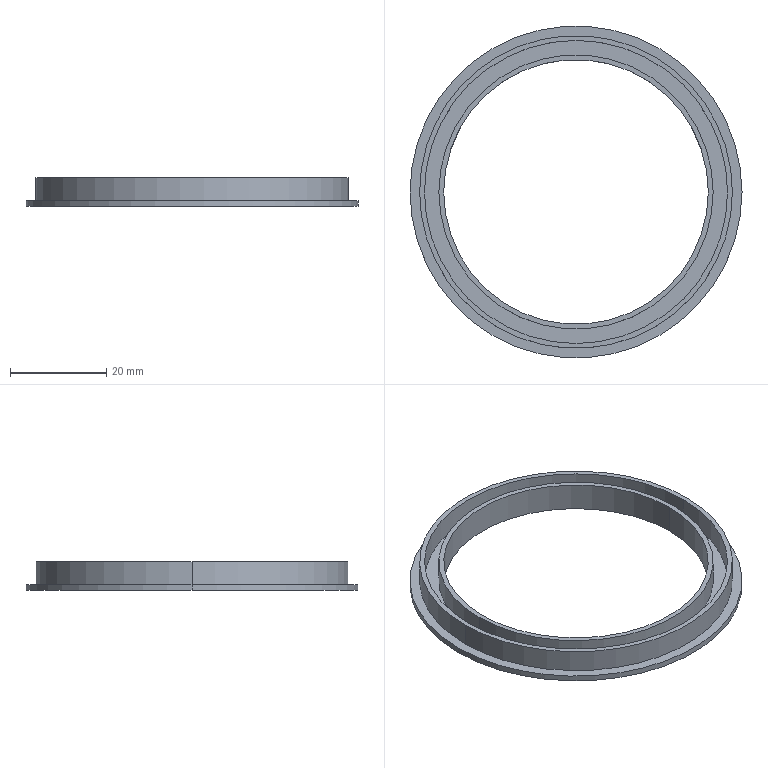Part | SolidWorks | features Extrusion 1, ICE 1 | 1 solid | 15 faces | box 69 x 69 x 6 mm | volume 3446 mm3 | cylinder 10 | plane 5 | commonest cylinder face diameters 55 x2 57 x2 63 x2 65 x2 69 x2
STEP:
#1=CARTESIAN_POINT('',(28.5,0.,6.));
#2=VERTEX_POINT('',#1);
#3=CARTESIAN_POINT('',(-28.5,0.,6.));
#4=VERTEX_POINT('',#3);
#5=CARTESIAN_POINT('',(0.,0.,6.));
#6=DIRECTION('',(0.,0.,1.));
#7=DIRECTION('',(1.,0.,0.));
#8=AXIS2_PLACEMENT_3D('',#5,#6,#7);
#9=CIRCLE('',#8,28.5);
#10=EDGE_CURVE('',#2,#4,#9,.T.);
#11=ORIENTED_EDGE('',*,*,#10,.F.);
#12=CARTESIAN_POINT('',(28.5,0.,1.2));
#13=VERTEX_POINT('',#12);
#14=CARTESIAN_POINT('',(28.5,0.,6.));
#15=DIRECTION('',(0.,0.,-1.));
#16=VECTOR('',#15,1000.);
#17=LINE('',#14,#16);
#18=EDGE_CURVE('',#2,#13,#17,.T.);
#19=ORIENTED_EDGE('',*,*,#18,.T.);
#20=CARTESIAN_POINT('',(-28.5,0.,1.2));
#21=VERTEX_POINT('',#20);
#22=CARTESIAN_POINT('',(0.,0.,1.2));
#23=DIRECTION('',(0.,0.,-1.));
#24=DIRECTION('',(1.,0.,0.));
#25=AXIS2_PLACEMENT_3D('',#22,#23,#24);
#26=CIRCLE('',#25,28.5);
#27=EDGE_CURVE('',#21,#13,#26,.T.);
#28=ORIENTED_EDGE('',*,*,#27,.F.);
#29=CARTESIAN_POINT('',(-28.5,0.,6.));
#30=DIRECTION('',(0.,0.,-1.));
#31=VECTOR('',#30,1000.);
#32=LINE('',#29,#31);
#33=EDGE_CURVE('',#4,#21,#32,.T.);
#34=ORIENTED_EDGE('',*,*,#33,.F.);
#35=EDGE_LOOP('',(#11,#19,#28,#34));
#36=FACE_OUTER_BOUND('',#35,.T.);
#37=CARTESIAN_POINT('',(0.,0.,6.));
#38=DIRECTION('',(0.,0.,-1.));
#39=DIRECTION('',(-1.,0.,0.));
#40=AXIS2_PLACEMENT_3D('',#37,#38,#39);
#41=CYLINDRICAL_SURFACE('',#40,28.5);
#42=ADVANCED_FACE('',(#36),#41,.T.);
#43=CARTESIAN_POINT('',(-27.5,0.,6.));
#44=VERTEX_POINT('',#43);
#45=CARTESIAN_POINT('',(27.5,0.,6.));
#46=VERTEX_POINT('',#45);
#47=CARTESIAN_POINT('',(0.,0.,6.));
#48=DIRECTION('',(0.,0.,1.));
#49=DIRECTION('',(1.,0.,0.));
#50=AXIS2_PLACEMENT_3D('',#47,#48,#49);
#51=CIRCLE('',#50,27.5);
#52=EDGE_CURVE('',#44,#46,#51,.T.);
#53=ORIENTED_EDGE('',*,*,#52,.T.);
#54=CARTESIAN_POINT('',(27.5,0.,0.));
#55=VERTEX_POINT('',#54);
#56=CARTESIAN_POINT('',(27.5,0.,1.2));
#57=DIRECTION('',(0.,0.,-1.));
#58=VECTOR('',#57,1000.);
#59=LINE('',#56,#58);
#60=EDGE_CURVE('',#46,#55,#59,.T.);
#61=ORIENTED_EDGE('',*,*,#60,.T.);
#62=CARTESIAN_POINT('',(-27.5,0.,0.));
#63=VERTEX_POINT('',#62);
#64=CARTESIAN_POINT('',(0.,0.,0.));
#65=DIRECTION('',(0.,0.,1.));
#66=DIRECTION('',(1.,0.,0.));
#67=AXIS2_PLACEMENT_3D('',#64,#65,#66);
#68=CIRCLE('',#67,27.5);
#69=EDGE_CURVE('',#63,#55,#68,.T.);
#70=ORIENTED_EDGE('',*,*,#69,.F.);
#71=CARTESIAN_POINT('',(-27.5,0.,1.2));
#72=DIRECTION('',(0.,0.,-1.));
#73=VECTOR('',#72,1000.);
#74=LINE('',#71,#73);
#75=EDGE_CURVE('',#44,#63,#74,.T.);
#76=ORIENTED_EDGE('',*,*,#75,.F.);
#77=EDGE_LOOP('',(#53,#61,#70,#76));
#78=FACE_OUTER_BOUND('',#77,.T.);
#79=CARTESIAN_POINT('',(0.,0.,1.2));
#80=DIRECTION('',(0.,0.,-1.));
#81=DIRECTION('',(-1.,0.,0.));
#82=AXIS2_PLACEMENT_3D('',#79,#80,#81);
#83=CYLINDRICAL_SURFACE('',#82,27.5);
#84=ADVANCED_FACE('',(#78),#83,.F.);
#85=CARTESIAN_POINT('',(34.5,0.,1.2));
#86=VERTEX_POINT('',#85);
#87=CARTESIAN_POINT('',(-34.5,0.,1.2));
#88=VERTEX_POINT('',#87);
#89=CARTESIAN_POINT('',(0.,0.,1.2));
#90=DIRECTION('',(0.,0.,1.));
#91=DIRECTION('',(1.,0.,0.));
#92=AXIS2_PLACEMENT_3D('',#89,#90,#91);
#93=CIRCLE('',#92,34.5);
#94=EDGE_CURVE('',#86,#88,#93,.T.);
#95=ORIENTED_EDGE('',*,*,#94,.F.);
#96=CARTESIAN_POINT('',(34.5,0.,0.));
#97=VERTEX_POINT('',#96);
#98=CARTESIAN_POINT('',(34.5,0.,1.2));
#99=DIRECTION('',(0.,0.,-1.));
#100=VECTOR('',#99,1000.);
#101=LINE('',#98,#100);
#102=EDGE_CURVE('',#86,#97,#101,.T.);
#103=ORIENTED_EDGE('',*,*,#102,.T.);
#104=CARTESIAN_POINT('',(-34.5,0.,0.));
#105=VERTEX_POINT('',#104);
#106=CARTESIAN_POINT('',(0.,0.,0.));
#107=DIRECTION('',(0.,0.,1.));
#108=DIRECTION('',(1.,0.,0.));
#109=AXIS2_PLACEMENT_3D('',#106,#107,#108);
#110=CIRCLE('',#109,34.5);
#111=EDGE_CURVE('',#97,#105,#110,.T.);
#112=ORIENTED_EDGE('',*,*,#111,.T.);
#113=CARTESIAN_POINT('',(-34.5,0.,1.2));
#114=DIRECTION('',(0.,0.,-1.));
#115=VECTOR('',#114,1000.);
#116=LINE('',#113,#115);
#117=EDGE_CURVE('',#88,#105,#116,.T.);
#118=ORIENTED_EDGE('',*,*,#117,.F.);
#119=EDGE_LOOP('',(#95,#103,#112,#118));
#120=FACE_OUTER_BOUND('',#119,.T.);
#121=CARTESIAN_POINT('',(0.,0.,1.2));
#122=DIRECTION('',(0.,0.,-1.));
#123=DIRECTION('',(-1.,0.,0.));
#124=AXIS2_PLACEMENT_3D('',#121,#122,#123);
#125=CYLINDRICAL_SURFACE('',#124,34.5);
#126=ADVANCED_FACE('',(#120),#125,.T.);
#127=CARTESIAN_POINT('',(32.5,0.,6.));
#128=VERTEX_POINT('',#127);
#129=CARTESIAN_POINT('',(-32.5,0.,6.));
#130=VERTEX_POINT('',#129);
#131=CARTESIAN_POINT('',(0.,0.,6.));
#132=DIRECTION('',(0.,0.,1.));
#133=DIRECTION('',(1.,0.,0.));
#134=AXIS2_PLACEMENT_3D('',#131,#132,#133);
#135=CIRCLE('',#134,32.5);
#136=EDGE_CURVE('',#128,#130,#135,.T.);
#137=ORIENTED_EDGE('',*,*,#136,.F.);
#138=CARTESIAN_POINT('',(32.5,0.,1.2));
#139=VERTEX_POINT('',#138);
#140=CARTESIAN_POINT('',(32.5,0.,6.));
#141=DIRECTION('',(0.,0.,-1.));
#142=VECTOR('',#141,1000.);
#143=LINE('',#140,#142);
#144=EDGE_CURVE('',#128,#139,#143,.T.);
#145=ORIENTED_EDGE('',*,*,#144,.T.);
#146=CARTESIAN_POINT('',(-32.5,0.,1.2));
#147=VERTEX_POINT('',#146);
#148=CARTESIAN_POINT('',(0.,0.,1.2));
#149=DIRECTION('',(0.,0.,1.));
#150=DIRECTION('',(1.,0.,0.));
#151=AXIS2_PLACEMENT_3D('',#148,#149,#150);
#152=CIRCLE('',#151,32.5);
#153=EDGE_CURVE('',#139,#147,#152,.T.);
#154=ORIENTED_EDGE('',*,*,#153,.T.);
#155=CARTESIAN_POINT('',(-32.5,0.,6.));
#156=DIRECTION('',(0.,0.,-1.));
#157=VECTOR('',#156,1000.);
#158=LINE('',#155,#157);
#159=EDGE_CURVE('',#130,#147,#158,.T.);
#160=ORIENTED_EDGE('',*,*,#159,.F.);
#161=EDGE_LOOP('',(#137,#145,#154,#160));
#162=FACE_OUTER_BOUND('',#161,.T.);
#163=CARTESIAN_POINT('',(0.,0.,6.));
#164=DIRECTION('',(0.,0.,-1.));
#165=DIRECTION('',(-1.,0.,0.));
#166=AXIS2_PLACEMENT_3D('',#163,#164,#165);
#167=CYLINDRICAL_SURFACE('',#166,32.5);
#168=ADVANCED_FACE('',(#162),#167,.T.);
#169=CARTESIAN_POINT('',(-31.5,0.,6.));
#170=VERTEX_POINT('',#169);
#171=CARTESIAN_POINT('',(31.5,0.,6.));
#172=VERTEX_POINT('',#171);
#173=CARTESIAN_POINT('',(0.,0.,6.));
#174=DIRECTION('',(0.,0.,1.));
#175=DIRECTION('',(1.,0.,0.));
#176=AXIS2_PLACEMENT_3D('',#173,#174,#175);
#177=CIRCLE('',#176,31.5);
#178=EDGE_CURVE('',#170,#172,#177,.T.);
#179=ORIENTED_EDGE('',*,*,#178,.T.);
#180=CARTESIAN_POINT('',(31.5,0.,1.2));
#181=VERTEX_POINT('',#180);
#182=CARTESIAN_POINT('',(31.5,0.,6.));
#183=DIRECTION('',(0.,0.,-1.));
#184=VECTOR('',#183,1000.);
#185=LINE('',#182,#184);
#186=EDGE_CURVE('',#172,#181,#185,.T.);
#187=ORIENTED_EDGE('',*,*,#186,.T.);
#188=CARTESIAN_POINT('',(-31.5,0.,1.2));
#189=VERTEX_POINT('',#188);
#190=CARTESIAN_POINT('',(0.,0.,1.2));
#191=DIRECTION('',(0.,0.,1.));
#192=DIRECTION('',(1.,0.,0.));
#193=AXIS2_PLACEMENT_3D('',#190,#191,#192);
#194=CIRCLE('',#193,31.5);
#195=EDGE_CURVE('',#189,#181,#194,.T.);
#196=ORIENTED_EDGE('',*,*,#195,.F.);
#197=CARTESIAN_POINT('',(-31.5,0.,6.));
#198=DIRECTION('',(0.,0.,-1.));
#199=VECTOR('',#198,1000.);
#200=LINE('',#197,#199);
#201=EDGE_CURVE('',#170,#189,#200,.T.);
#202=ORIENTED_EDGE('',*,*,#201,.F.);
#203=EDGE_LOOP('',(#179,#187,#196,#202));
#204=FACE_OUTER_BOUND('',#203,.T.);
#205=CARTESIAN_POINT('',(0.,0.,6.));
#206=DIRECTION('',(0.,0.,-1.));
#207=DIRECTION('',(-1.,0.,0.));
#208=AXIS2_PLACEMENT_3D('',#205,#206,#207);
#209=CYLINDRICAL_SURFACE('',#208,31.5);
#210=ADVANCED_FACE('',(#204),#209,.F.);
#211=ORIENTED_EDGE('',*,*,#186,.F.);
#212=CARTESIAN_POINT('',(0.,0.,6.));
#213=DIRECTION('',(0.,0.,1.));
#214=DIRECTION('',(1.,0.,0.));
#215=AXIS2_PLACEMENT_3D('',#212,#213,#214);
#216=CIRCLE('',#215,31.5);
#217=EDGE_CURVE('',#172,#170,#216,.T.);
#218=ORIENTED_EDGE('',*,*,#217,.T.);
#219=ORIENTED_EDGE('',*,*,#201,.T.);
#220=CARTESIAN_POINT('',(0.,0.,1.2));
#221=DIRECTION('',(0.,0.,1.));
#222=DIRECTION('',(1.,0.,0.));
#223=AXIS2_PLACEMENT_3D('',#220,#221,#222);
#224=CIRCLE('',#223,31.5);
#225=EDGE_CURVE('',#181,#189,#224,.T.);
#226=ORIENTED_EDGE('',*,*,#225,.F.);
#227=EDGE_LOOP('',(#211,#218,#219,#226));
#228=FACE_OUTER_BOUND('',#227,.T.);
#229=CARTESIAN_POINT('',(0.,0.,6.));
#230=DIRECTION('',(0.,0.,-1.));
#231=DIRECTION('',(-1.,0.,0.));
#232=AXIS2_PLACEMENT_3D('',#229,#230,#231);
#233=CYLINDRICAL_SURFACE('',#232,31.5);
#234=ADVANCED_FACE('',(#228),#233,.F.);
#235=ORIENTED_EDGE('',*,*,#144,.F.);
#236=CARTESIAN_POINT('',(0.,0.,6.));
#237=DIRECTION('',(0.,0.,1.));
#238=DIRECTION('',(1.,0.,0.));
#239=AXIS2_PLACEMENT_3D('',#236,#237,#238);
#240=CIRCLE('',#239,32.5);
#241=EDGE_CURVE('',#130,#128,#240,.T.);
#242=ORIENTED_EDGE('',*,*,#241,.F.);
#243=ORIENTED_EDGE('',*,*,#159,.T.);
#244=CARTESIAN_POINT('',(0.,0.,1.2));
#245=DIRECTION('',(0.,0.,1.));
#246=DIRECTION('',(1.,0.,0.));
#247=AXIS2_PLACEMENT_3D('',#244,#245,#246);
#248=CIRCLE('',#247,32.5);
#249=EDGE_CURVE('',#147,#139,#248,.T.);
#250=ORIENTED_EDGE('',*,*,#249,.T.);
#251=EDGE_LOOP('',(#235,#242,#243,#250));
#252=FACE_OUTER_BOUND('',#251,.T.);
#253=CARTESIAN_POINT('',(0.,0.,6.));
#254=DIRECTION('',(0.,0.,-1.));
#255=DIRECTION('',(-1.,0.,0.));
#256=AXIS2_PLACEMENT_3D('',#253,#254,#255);
#257=CYLINDRICAL_SURFACE('',#256,32.5);
#258=ADVANCED_FACE('',(#252),#257,.T.);
#259=ORIENTED_EDGE('',*,*,#178,.F.);
#260=ORIENTED_EDGE('',*,*,#217,.F.);
#261=EDGE_LOOP('',(#259,#260));
#262=FACE_BOUND('',#261,.T.);
#263=ORIENTED_EDGE('',*,*,#241,.T.);
#264=ORIENTED_EDGE('',*,*,#136,.T.);
#265=EDGE_LOOP('',(#263,#264));
#266=FACE_OUTER_BOUND('',#265,.T.);
#267=CARTESIAN_POINT('',(0.,0.,6.));
#268=DIRECTION('',(0.,0.,1.));
#269=DIRECTION('',(1.,0.,0.));
#270=AXIS2_PLACEMENT_3D('',#267,#268,#269);
#271=PLANE('',#270);
#272=ADVANCED_FACE('',(#262,#266),#271,.T.);
#273=ORIENTED_EDGE('',*,*,#249,.F.);
#274=ORIENTED_EDGE('',*,*,#153,.F.);
#275=EDGE_LOOP('',(#273,#274));
#276=FACE_BOUND('',#275,.T.);
#277=CARTESIAN_POINT('',(0.,0.,1.2));
#278=DIRECTION('',(0.,0.,1.));
#279=DIRECTION('',(1.,0.,0.));
#280=AXIS2_PLACEMENT_3D('',#277,#278,#279);
#281=CIRCLE('',#280,34.5);
#282=EDGE_CURVE('',#88,#86,#281,.T.);
#283=ORIENTED_EDGE('',*,*,#282,.T.);
#284=ORIENTED_EDGE('',*,*,#94,.T.);
#285=EDGE_LOOP('',(#283,#284));
#286=FACE_OUTER_BOUND('',#285,.T.);
#287=CARTESIAN_POINT('',(0.,0.,1.2));
#288=DIRECTION('',(0.,0.,1.));
#289=DIRECTION('',(1.,0.,0.));
#290=AXIS2_PLACEMENT_3D('',#287,#288,#289);
#291=PLANE('',#290);
#292=ADVANCED_FACE('',(#276,#286),#291,.T.);
#293=ORIENTED_EDGE('',*,*,#102,.F.);
#294=ORIENTED_EDGE('',*,*,#282,.F.);
#295=ORIENTED_EDGE('',*,*,#117,.T.);
#296=CARTESIAN_POINT('',(0.,0.,0.));
#297=DIRECTION('',(0.,0.,1.));
#298=DIRECTION('',(1.,0.,0.));
#299=AXIS2_PLACEMENT_3D('',#296,#297,#298);
#300=CIRCLE('',#299,34.5);
#301=EDGE_CURVE('',#105,#97,#300,.T.);
#302=ORIENTED_EDGE('',*,*,#301,.T.);
#303=EDGE_LOOP('',(#293,#294,#295,#302));
#304=FACE_OUTER_BOUND('',#303,.T.);
#305=CARTESIAN_POINT('',(0.,0.,1.2));
#306=DIRECTION('',(0.,0.,-1.));
#307=DIRECTION('',(-1.,0.,0.));
#308=AXIS2_PLACEMENT_3D('',#305,#306,#307);
#309=CYLINDRICAL_SURFACE('',#308,34.5);
#310=ADVANCED_FACE('',(#304),#309,.T.);
#311=ORIENTED_EDGE('',*,*,#301,.F.);
#312=ORIENTED_EDGE('',*,*,#111,.F.);
#313=EDGE_LOOP('',(#311,#312));
#314=FACE_OUTER_BOUND('',#313,.T.);
#315=ORIENTED_EDGE('',*,*,#69,.T.);
#316=CARTESIAN_POINT('',(0.,0.,0.));
#317=DIRECTION('',(0.,0.,1.));
#318=DIRECTION('',(1.,0.,0.));
#319=AXIS2_PLACEMENT_3D('',#316,#317,#318);
#320=CIRCLE('',#319,27.5);
#321=EDGE_CURVE('',#55,#63,#320,.T.);
#322=ORIENTED_EDGE('',*,*,#321,.T.);
#323=EDGE_LOOP('',(#315,#322));
#324=FACE_BOUND('',#323,.T.);
#325=CARTESIAN_POINT('',(0.,0.,0.));
#326=DIRECTION('',(0.,0.,1.));
#327=DIRECTION('',(1.,0.,0.));
#328=AXIS2_PLACEMENT_3D('',#325,#326,#327);
#329=PLANE('',#328);
#330=ADVANCED_FACE('',(#314,#324),#329,.F.);
#331=ORIENTED_EDGE('',*,*,#27,.T.);
#332=CARTESIAN_POINT('',(0.,0.,1.2));
#333=DIRECTION('',(0.,0.,-1.));
#334=DIRECTION('',(1.,0.,0.));
#335=AXIS2_PLACEMENT_3D('',#332,#333,#334);
#336=CIRCLE('',#335,28.5);
#337=EDGE_CURVE('',#13,#21,#336,.T.);
#338=ORIENTED_EDGE('',*,*,#337,.T.);
#339=EDGE_LOOP('',(#331,#338));
#340=FACE_BOUND('',#339,.T.);
#341=ORIENTED_EDGE('',*,*,#195,.T.);
#342=ORIENTED_EDGE('',*,*,#225,.T.);
#343=EDGE_LOOP('',(#341,#342));
#344=FACE_OUTER_BOUND('',#343,.T.);
#345=CARTESIAN_POINT('',(0.,0.,1.2));
#346=DIRECTION('',(0.,0.,1.));
#347=DIRECTION('',(1.,0.,0.));
#348=AXIS2_PLACEMENT_3D('',#345,#346,#347);
#349=PLANE('',#348);
#350=ADVANCED_FACE('',(#340,#344),#349,.T.);
#351=ORIENTED_EDGE('',*,*,#60,.F.);
#352=CARTESIAN_POINT('',(0.,0.,6.));
#353=DIRECTION('',(0.,0.,1.));
#354=DIRECTION('',(1.,0.,0.));
#355=AXIS2_PLACEMENT_3D('',#352,#353,#354);
#356=CIRCLE('',#355,27.5);
#357=EDGE_CURVE('',#46,#44,#356,.T.);
#358=ORIENTED_EDGE('',*,*,#357,.T.);
#359=ORIENTED_EDGE('',*,*,#75,.T.);
#360=ORIENTED_EDGE('',*,*,#321,.F.);
#361=EDGE_LOOP('',(#351,#358,#359,#360));
#362=FACE_OUTER_BOUND('',#361,.T.);
#363=CARTESIAN_POINT('',(0.,0.,1.2));
#364=DIRECTION('',(0.,0.,-1.));
#365=DIRECTION('',(-1.,0.,0.));
#366=AXIS2_PLACEMENT_3D('',#363,#364,#365);
#367=CYLINDRICAL_SURFACE('',#366,27.5);
#368=ADVANCED_FACE('',(#362),#367,.F.);
#369=ORIENTED_EDGE('',*,*,#18,.F.);
#370=CARTESIAN_POINT('',(0.,0.,6.));
#371=DIRECTION('',(0.,0.,1.));
#372=DIRECTION('',(1.,0.,0.));
#373=AXIS2_PLACEMENT_3D('',#370,#371,#372);
#374=CIRCLE('',#373,28.5);
#375=EDGE_CURVE('',#4,#2,#374,.T.);
#376=ORIENTED_EDGE('',*,*,#375,.F.);
#377=ORIENTED_EDGE('',*,*,#33,.T.);
#378=ORIENTED_EDGE('',*,*,#337,.F.);
#379=EDGE_LOOP('',(#369,#376,#377,#378));
#380=FACE_OUTER_BOUND('',#379,.T.);
#381=CARTESIAN_POINT('',(0.,0.,6.));
#382=DIRECTION('',(0.,0.,-1.));
#383=DIRECTION('',(-1.,0.,0.));
#384=AXIS2_PLACEMENT_3D('',#381,#382,#383);
#385=CYLINDRICAL_SURFACE('',#384,28.5);
#386=ADVANCED_FACE('',(#380),#385,.T.);
#387=ORIENTED_EDGE('',*,*,#52,.F.);
#388=ORIENTED_EDGE('',*,*,#357,.F.);
#389=EDGE_LOOP('',(#387,#388));
#390=FACE_BOUND('',#389,.T.);
#391=ORIENTED_EDGE('',*,*,#375,.T.);
#392=ORIENTED_EDGE('',*,*,#10,.T.);
#393=EDGE_LOOP('',(#391,#392));
#394=FACE_OUTER_BOUND('',#393,.T.);
#395=CARTESIAN_POINT('',(0.,0.,6.));
#396=DIRECTION('',(0.,0.,1.));
#397=DIRECTION('',(1.,0.,0.));
#398=AXIS2_PLACEMENT_3D('',#395,#396,#397);
#399=PLANE('',#398);
#400=ADVANCED_FACE('',(#390,#394),#399,.T.);
#401=CLOSED_SHELL('',(#42,#84,#126,#168,#210,#234,#258,#272,#292,#310,#330,#350,#368,#386,#400));
#402=MANIFOLD_SOLID_BREP('',#401);
#403=CARTESIAN_POINT('',(0.,0.,0.));
#404=DIRECTION('',(0.,0.,1.));
#405=DIRECTION('',(1.,0.,0.));
#406=AXIS2_PLACEMENT_3D('',#403,#404,#405);
#407=(LENGTH_UNIT()NAMED_UNIT(*)SI_UNIT(.MILLI.,.METRE.));
#408=UNCERTAINTY_MEASURE_WITH_UNIT(LENGTH_MEASURE(0.00001),#407,'','');
#409=(NAMED_UNIT(*)PLANE_ANGLE_UNIT()SI_UNIT($,.RADIAN.));
#410=(NAMED_UNIT(*)SI_UNIT($,.STERADIAN.)SOLID_ANGLE_UNIT());
#411=(GEOMETRIC_REPRESENTATION_CONTEXT(3)GLOBAL_UNCERTAINTY_ASSIGNED_CONTEXT((#408))GLOBAL_UNIT_ASSIGNED_CONTEXT((#407,#409,#410))REPRESENTATION_CONTEXT('',''));
#412=ADVANCED_BREP_SHAPE_REPRESENTATION('',(#402,#406),#411);